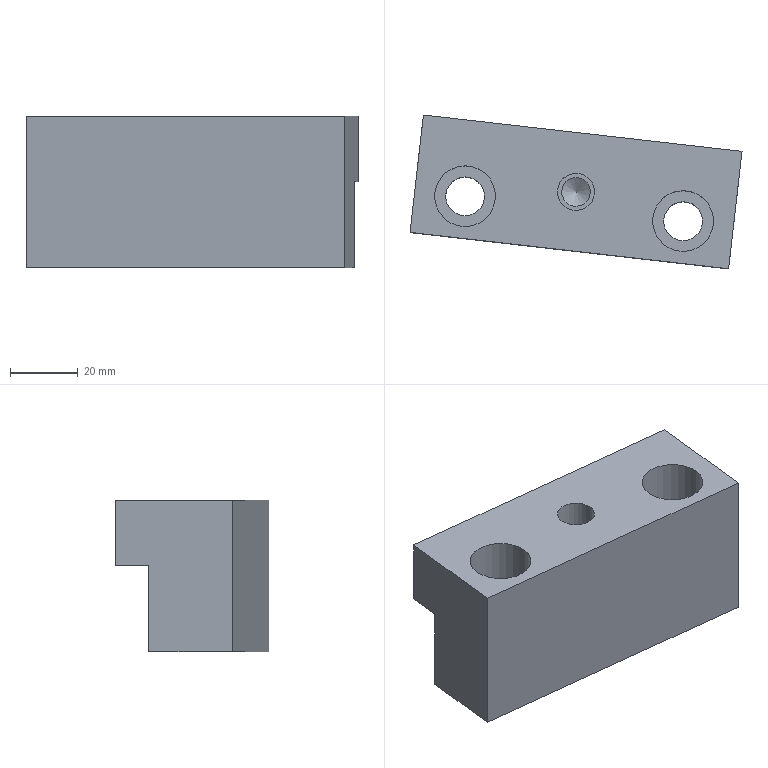Part | NX | features XQ 2 | 1 solid | 18 faces | box 98.351 x 45.529 x 45 mm | volume 108255 mm3 | plane 11 | cylinder 6 | cone 1 | commonest cylinder face diameters 11.5 x2 18 x2 8.5 x1 11 x1
STEP:
#1=CARTESIAN_POINT('',(3233.637,-396.68,-143.));
#2=VERTEX_POINT('',#1);
#3=CARTESIAN_POINT('',(3230.807,-421.519,-143.));
#4=VERTEX_POINT('',#3);
#5=CARTESIAN_POINT('',(3233.637,-396.68,-143.));
#6=DIRECTION('',(-0.1132,-0.9936,0.));
#7=VECTOR('',#6,1000.);
#8=LINE('',#5,#7);
#9=EDGE_CURVE('',#2,#4,#8,.T.);
#10=ORIENTED_EDGE('',*,*,#9,.F.);
#11=CARTESIAN_POINT('',(3328.026,-407.434,-143.));
#12=VERTEX_POINT('',#11);
#13=CARTESIAN_POINT('',(1661.613,-217.57,-143.));
#14=DIRECTION('',(-0.9936,0.1132,0.));
#15=VECTOR('',#14,1000.);
#16=LINE('',#13,#15);
#17=EDGE_CURVE('',#12,#2,#16,.T.);
#18=ORIENTED_EDGE('',*,*,#17,.F.);
#19=CARTESIAN_POINT('',(3325.196,-432.273,-143.));
#20=VERTEX_POINT('',#19);
#21=CARTESIAN_POINT('',(3342.856,-277.276,-143.));
#22=DIRECTION('',(-0.1132,-0.9936,0.));
#23=VECTOR('',#22,1000.);
#24=LINE('',#21,#23);
#25=EDGE_CURVE('',#12,#20,#24,.T.);
#26=ORIENTED_EDGE('',*,*,#25,.T.);
#27=CARTESIAN_POINT('',(1658.783,-242.409,-143.));
#28=DIRECTION('',(-0.9936,0.1132,0.));
#29=VECTOR('',#28,1000.);
#30=LINE('',#27,#29);
#31=EDGE_CURVE('',#20,#4,#30,.T.);
#32=ORIENTED_EDGE('',*,*,#31,.T.);
#33=EDGE_LOOP('',(#10,#18,#26,#32));
#34=FACE_BOUND('',#33,.T.);
#35=CARTESIAN_POINT('',(3311.708,-412.406,-143.));
#36=VERTEX_POINT('',#35);
#37=CARTESIAN_POINT('',(3311.708,-418.156,-143.));
#38=DIRECTION('',(0.,0.,-1.));
#39=DIRECTION('',(0.,1.,0.));
#40=AXIS2_PLACEMENT_3D('',#37,#38,#39);
#41=CIRCLE('',#40,5.75);
#42=EDGE_CURVE('',#36,#36,#41,.T.);
#43=ORIENTED_EDGE('',*,*,#42,.F.);
#44=EDGE_LOOP('',(#43));
#45=FACE_BOUND('',#44,.T.);
#46=CARTESIAN_POINT('',(3247.125,-405.047,-143.));
#47=VERTEX_POINT('',#46);
#48=CARTESIAN_POINT('',(3247.125,-410.797,-143.));
#49=DIRECTION('',(0.,0.,1.));
#50=DIRECTION('',(0.,1.,0.));
#51=AXIS2_PLACEMENT_3D('',#48,#49,#50);
#52=CIRCLE('',#51,5.75);
#53=EDGE_CURVE('',#47,#47,#52,.T.);
#54=ORIENTED_EDGE('',*,*,#53,.T.);
#55=EDGE_LOOP('',(#54));
#56=FACE_BOUND('',#55,.T.);
#57=CARTESIAN_POINT('',(1661.613,-217.57,-143.));
#58=DIRECTION('',(0.,0.,1.));
#59=DIRECTION('',(-0.9936,0.1132,0.));
#60=AXIS2_PLACEMENT_3D('',#57,#58,#59);
#61=PLANE('',#60);
#62=ADVANCED_FACE('',(#34,#45,#56),#61,.F.);
#63=CARTESIAN_POINT('',(3285.256,-411.071,-98.));
#64=VERTEX_POINT('',#63);
#65=CARTESIAN_POINT('',(3279.983,-409.509,-98.));
#66=DIRECTION('',(0.,0.,1.));
#67=DIRECTION('',(0.9588,-0.284,0.));
#68=AXIS2_PLACEMENT_3D('',#65,#66,#67);
#69=CIRCLE('',#68,5.5);
#70=EDGE_CURVE('',#64,#64,#69,.T.);
#71=ORIENTED_EDGE('',*,*,#70,.F.);
#72=EDGE_LOOP('',(#71));
#73=FACE_BOUND('',#72,.T.);
#74=CARTESIAN_POINT('',(3329.158,-397.498,-98.));
#75=VERTEX_POINT('',#74);
#76=CARTESIAN_POINT('',(3234.769,-386.744,-98.));
#77=VERTEX_POINT('',#76);
#78=CARTESIAN_POINT('',(3270.538,-390.819,-98.));
#79=DIRECTION('',(-0.9936,0.1132,0.));
#80=VECTOR('',#79,1000.);
#81=LINE('',#78,#80);
#82=EDGE_CURVE('',#75,#77,#81,.T.);
#83=ORIENTED_EDGE('',*,*,#82,.T.);
#84=CARTESIAN_POINT('',(3230.807,-421.519,-98.));
#85=VERTEX_POINT('',#84);
#86=CARTESIAN_POINT('',(3252.077,-234.832,-98.));
#87=DIRECTION('',(-0.1132,-0.9936,0.));
#88=VECTOR('',#87,1000.);
#89=LINE('',#86,#88);
#90=EDGE_CURVE('',#77,#85,#89,.T.);
#91=ORIENTED_EDGE('',*,*,#90,.T.);
#92=CARTESIAN_POINT('',(3325.196,-432.273,-98.));
#93=VERTEX_POINT('',#92);
#94=CARTESIAN_POINT('',(3287.44,-427.972,-98.));
#95=DIRECTION('',(-0.9936,0.1132,0.));
#96=VECTOR('',#95,1000.);
#97=LINE('',#94,#96);
#98=EDGE_CURVE('',#93,#85,#97,.T.);
#99=ORIENTED_EDGE('',*,*,#98,.F.);
#100=CARTESIAN_POINT('',(3346.466,-245.587,-98.));
#101=DIRECTION('',(-0.1132,-0.9936,0.));
#102=VECTOR('',#101,1000.);
#103=LINE('',#100,#102);
#104=EDGE_CURVE('',#75,#93,#103,.T.);
#105=ORIENTED_EDGE('',*,*,#104,.F.);
#106=EDGE_LOOP('',(#83,#91,#99,#105));
#107=FACE_BOUND('',#106,.T.);
#108=CARTESIAN_POINT('',(3311.708,-409.156,-98.));
#109=VERTEX_POINT('',#108);
#110=CARTESIAN_POINT('',(3311.708,-418.156,-98.));
#111=DIRECTION('',(0.,0.,1.));
#112=DIRECTION('',(0.,1.,0.));
#113=AXIS2_PLACEMENT_3D('',#110,#111,#112);
#114=CIRCLE('',#113,9.);
#115=EDGE_CURVE('',#109,#109,#114,.T.);
#116=ORIENTED_EDGE('',*,*,#115,.F.);
#117=EDGE_LOOP('',(#116));
#118=FACE_BOUND('',#117,.T.);
#119=CARTESIAN_POINT('',(3247.125,-401.797,-98.));
#120=VERTEX_POINT('',#119);
#121=CARTESIAN_POINT('',(3247.125,-410.797,-98.));
#122=DIRECTION('',(0.,0.,-1.));
#123=DIRECTION('',(0.,1.,0.));
#124=AXIS2_PLACEMENT_3D('',#121,#122,#123);
#125=CIRCLE('',#124,9.);
#126=EDGE_CURVE('',#120,#120,#125,.T.);
#127=ORIENTED_EDGE('',*,*,#126,.T.);
#128=EDGE_LOOP('',(#127));
#129=FACE_BOUND('',#128,.T.);
#130=CARTESIAN_POINT('',(2553.344,-155.222,-98.));
#131=DIRECTION('',(0.,0.,1.));
#132=DIRECTION('',(0.9588,-0.284,0.));
#133=AXIS2_PLACEMENT_3D('',#130,#131,#132);
#134=PLANE('',#133);
#135=ADVANCED_FACE('',(#73,#107,#118,#129),#134,.T.);
#136=CARTESIAN_POINT('',(3234.769,-386.744,-117.5));
#137=VERTEX_POINT('',#136);
#138=CARTESIAN_POINT('',(3233.637,-396.68,-117.5));
#139=VERTEX_POINT('',#138);
#140=CARTESIAN_POINT('',(3233.637,-396.68,-117.5));
#141=DIRECTION('',(-0.1132,-0.9936,0.));
#142=VECTOR('',#141,1000.);
#143=LINE('',#140,#142);
#144=EDGE_CURVE('',#137,#139,#143,.T.);
#145=ORIENTED_EDGE('',*,*,#144,.T.);
#146=CARTESIAN_POINT('',(3233.637,-396.68,-128.027));
#147=DIRECTION('',(0.,0.,1.));
#148=VECTOR('',#147,1000.);
#149=LINE('',#146,#148);
#150=EDGE_CURVE('',#2,#139,#149,.T.);
#151=ORIENTED_EDGE('',*,*,#150,.F.);
#152=ORIENTED_EDGE('',*,*,#9,.T.);
#153=CARTESIAN_POINT('',(3230.807,-421.519,-128.027));
#154=DIRECTION('',(0.,0.,1.));
#155=VECTOR('',#154,1000.);
#156=LINE('',#153,#155);
#157=EDGE_CURVE('',#4,#85,#156,.T.);
#158=ORIENTED_EDGE('',*,*,#157,.T.);
#159=ORIENTED_EDGE('',*,*,#90,.F.);
#160=CARTESIAN_POINT('',(3234.769,-386.744,-128.027));
#161=DIRECTION('',(0.,0.,1.));
#162=VECTOR('',#161,1000.);
#163=LINE('',#160,#162);
#164=EDGE_CURVE('',#137,#77,#163,.T.);
#165=ORIENTED_EDGE('',*,*,#164,.F.);
#166=EDGE_LOOP('',(#145,#151,#152,#158,#159,#165));
#167=FACE_BOUND('',#166,.T.);
#168=CARTESIAN_POINT('',(3233.637,-396.68,-128.027));
#169=DIRECTION('',(0.9936,-0.1132,0.));
#170=DIRECTION('',(0.,0.,1.));
#171=AXIS2_PLACEMENT_3D('',#168,#169,#170);
#172=PLANE('',#171);
#173=ADVANCED_FACE('',(#167),#172,.F.);
#174=CARTESIAN_POINT('',(3329.158,-397.498,-117.5));
#175=VERTEX_POINT('',#174);
#176=CARTESIAN_POINT('',(3329.158,-397.498,-118.));
#177=DIRECTION('',(0.,0.,1.));
#178=VECTOR('',#177,1000.);
#179=LINE('',#176,#178);
#180=EDGE_CURVE('',#175,#75,#179,.T.);
#181=ORIENTED_EDGE('',*,*,#180,.T.);
#182=ORIENTED_EDGE('',*,*,#104,.T.);
#183=CARTESIAN_POINT('',(3325.196,-432.273,-118.));
#184=DIRECTION('',(0.,0.,1.));
#185=VECTOR('',#184,1000.);
#186=LINE('',#183,#185);
#187=EDGE_CURVE('',#20,#93,#186,.T.);
#188=ORIENTED_EDGE('',*,*,#187,.F.);
#189=ORIENTED_EDGE('',*,*,#25,.F.);
#190=CARTESIAN_POINT('',(3328.026,-407.434,-117.5));
#191=VERTEX_POINT('',#190);
#192=CARTESIAN_POINT('',(3328.026,-407.434,-118.));
#193=DIRECTION('',(0.,0.,1.));
#194=VECTOR('',#193,1000.);
#195=LINE('',#192,#194);
#196=EDGE_CURVE('',#12,#191,#195,.T.);
#197=ORIENTED_EDGE('',*,*,#196,.T.);
#198=CARTESIAN_POINT('',(3338.113,-318.901,-117.5));
#199=DIRECTION('',(-0.1132,-0.9936,0.));
#200=VECTOR('',#199,1000.);
#201=LINE('',#198,#200);
#202=EDGE_CURVE('',#175,#191,#201,.T.);
#203=ORIENTED_EDGE('',*,*,#202,.F.);
#204=EDGE_LOOP('',(#181,#182,#188,#189,#197,#203));
#205=FACE_BOUND('',#204,.T.);
#206=CARTESIAN_POINT('',(3342.856,-277.276,-118.));
#207=DIRECTION('',(-0.9936,0.1132,0.));
#208=DIRECTION('',(-0.1132,-0.9936,0.));
#209=AXIS2_PLACEMENT_3D('',#206,#207,#208);
#210=PLANE('',#209);
#211=ADVANCED_FACE('',(#205),#210,.F.);
#212=ORIENTED_EDGE('',*,*,#187,.T.);
#213=ORIENTED_EDGE('',*,*,#98,.T.);
#214=ORIENTED_EDGE('',*,*,#157,.F.);
#215=ORIENTED_EDGE('',*,*,#31,.F.);
#216=EDGE_LOOP('',(#212,#213,#214,#215));
#217=FACE_BOUND('',#216,.T.);
#218=CARTESIAN_POINT('',(3287.44,-427.972,-88.563));
#219=DIRECTION('',(-0.1132,-0.9936,0.));
#220=DIRECTION('',(0.9936,-0.1132,0.));
#221=AXIS2_PLACEMENT_3D('',#218,#219,#220);
#222=PLANE('',#221);
#223=ADVANCED_FACE('',(#217),#222,.T.);
#224=CARTESIAN_POINT('',(2534.904,-317.069,-117.5));
#225=DIRECTION('',(-0.9936,0.1132,0.));
#226=VECTOR('',#225,1000.);
#227=LINE('',#224,#226);
#228=EDGE_CURVE('',#191,#139,#227,.T.);
#229=ORIENTED_EDGE('',*,*,#228,.F.);
#230=ORIENTED_EDGE('',*,*,#196,.F.);
#231=ORIENTED_EDGE('',*,*,#17,.T.);
#232=ORIENTED_EDGE('',*,*,#150,.T.);
#233=EDGE_LOOP('',(#229,#230,#231,#232));
#234=FACE_BOUND('',#233,.T.);
#235=CARTESIAN_POINT('',(3290.27,-403.132,-88.563));
#236=DIRECTION('',(-0.1132,-0.9936,0.));
#237=DIRECTION('',(0.9936,-0.1132,0.));
#238=AXIS2_PLACEMENT_3D('',#235,#236,#237);
#239=PLANE('',#238);
#240=ADVANCED_FACE('',(#234),#239,.F.);
#241=CARTESIAN_POINT('',(3270.538,-390.819,-117.5));
#242=DIRECTION('',(0.9936,-0.1132,0.));
#243=VECTOR('',#242,1000.);
#244=LINE('',#241,#243);
#245=EDGE_CURVE('',#137,#175,#244,.T.);
#246=ORIENTED_EDGE('',*,*,#245,.T.);
#247=ORIENTED_EDGE('',*,*,#202,.T.);
#248=ORIENTED_EDGE('',*,*,#228,.T.);
#249=ORIENTED_EDGE('',*,*,#144,.F.);
#250=EDGE_LOOP('',(#246,#247,#248,#249));
#251=FACE_BOUND('',#250,.T.);
#252=CARTESIAN_POINT('',(2544.991,-228.537,-117.5));
#253=DIRECTION('',(0.,0.,1.));
#254=DIRECTION('',(0.9981,0.06105,0.));
#255=AXIS2_PLACEMENT_3D('',#252,#253,#254);
#256=PLANE('',#255);
#257=ADVANCED_FACE('',(#251),#256,.F.);
#258=ORIENTED_EDGE('',*,*,#164,.T.);
#259=ORIENTED_EDGE('',*,*,#82,.F.);
#260=ORIENTED_EDGE('',*,*,#180,.F.);
#261=ORIENTED_EDGE('',*,*,#245,.F.);
#262=EDGE_LOOP('',(#258,#259,#260,#261));
#263=FACE_BOUND('',#262,.T.);
#264=CARTESIAN_POINT('',(3270.538,-390.819,-81.063));
#265=DIRECTION('',(-0.1132,-0.9936,0.));
#266=DIRECTION('',(0.9936,-0.1132,0.));
#267=AXIS2_PLACEMENT_3D('',#264,#265,#266);
#268=PLANE('',#267);
#269=ADVANCED_FACE('',(#263),#268,.F.);
#270=CARTESIAN_POINT('',(3311.708,-423.906,-118.));
#271=VERTEX_POINT('',#270);
#272=CARTESIAN_POINT('',(3311.708,-418.156,-118.));
#273=DIRECTION('',(0.,0.,1.));
#274=DIRECTION('',(0.,-1.,0.));
#275=AXIS2_PLACEMENT_3D('',#272,#273,#274);
#276=CIRCLE('',#275,5.75);
#277=EDGE_CURVE('',#271,#271,#276,.T.);
#278=ORIENTED_EDGE('',*,*,#277,.T.);
#279=EDGE_LOOP('',(#278));
#280=FACE_BOUND('',#279,.T.);
#281=ORIENTED_EDGE('',*,*,#42,.T.);
#282=EDGE_LOOP('',(#281));
#283=FACE_BOUND('',#282,.T.);
#284=CARTESIAN_POINT('',(3311.708,-418.156,-103.));
#285=DIRECTION('',(0.,0.,-1.));
#286=DIRECTION('',(-0.9981,-0.06105,0.));
#287=AXIS2_PLACEMENT_3D('',#284,#285,#286);
#288=CYLINDRICAL_SURFACE('',#287,5.75);
#289=ADVANCED_FACE('',(#280,#283),#288,.F.);
#290=ORIENTED_EDGE('',*,*,#277,.F.);
#291=EDGE_LOOP('',(#290));
#292=FACE_BOUND('',#291,.T.);
#293=CARTESIAN_POINT('',(3311.708,-427.156,-118.));
#294=VERTEX_POINT('',#293);
#295=CARTESIAN_POINT('',(3311.708,-418.156,-118.));
#296=DIRECTION('',(0.,0.,1.));
#297=DIRECTION('',(0.,-1.,0.));
#298=AXIS2_PLACEMENT_3D('',#295,#296,#297);
#299=CIRCLE('',#298,9.);
#300=EDGE_CURVE('',#294,#294,#299,.T.);
#301=ORIENTED_EDGE('',*,*,#300,.T.);
#302=EDGE_LOOP('',(#301));
#303=FACE_BOUND('',#302,.T.);
#304=CARTESIAN_POINT('',(3311.708,-418.156,-118.));
#305=DIRECTION('',(0.,0.,-1.));
#306=DIRECTION('',(0.9981,0.06105,0.));
#307=AXIS2_PLACEMENT_3D('',#304,#305,#306);
#308=PLANE('',#307);
#309=ADVANCED_FACE('',(#292,#303),#308,.F.);
#310=ORIENTED_EDGE('',*,*,#300,.F.);
#311=EDGE_LOOP('',(#310));
#312=FACE_BOUND('',#311,.T.);
#313=ORIENTED_EDGE('',*,*,#115,.T.);
#314=EDGE_LOOP('',(#313));
#315=FACE_BOUND('',#314,.T.);
#316=CARTESIAN_POINT('',(3311.708,-418.156,-103.));
#317=DIRECTION('',(0.,0.,-1.));
#318=DIRECTION('',(-0.9981,-0.06105,0.));
#319=AXIS2_PLACEMENT_3D('',#316,#317,#318);
#320=CYLINDRICAL_SURFACE('',#319,9.);
#321=ADVANCED_FACE('',(#312,#315),#320,.F.);
#322=CARTESIAN_POINT('',(3247.125,-416.547,-118.));
#323=VERTEX_POINT('',#322);
#324=CARTESIAN_POINT('',(3247.125,-410.797,-118.));
#325=DIRECTION('',(0.,0.,-1.));
#326=DIRECTION('',(0.,-1.,0.));
#327=AXIS2_PLACEMENT_3D('',#324,#325,#326);
#328=CIRCLE('',#327,5.75);
#329=EDGE_CURVE('',#323,#323,#328,.T.);
#330=ORIENTED_EDGE('',*,*,#329,.F.);
#331=EDGE_LOOP('',(#330));
#332=FACE_BOUND('',#331,.T.);
#333=ORIENTED_EDGE('',*,*,#53,.F.);
#334=EDGE_LOOP('',(#333));
#335=FACE_BOUND('',#334,.T.);
#336=CARTESIAN_POINT('',(3247.125,-410.797,-103.));
#337=DIRECTION('',(0.,0.,-1.));
#338=DIRECTION('',(0.9588,-0.284,0.));
#339=AXIS2_PLACEMENT_3D('',#336,#337,#338);
#340=CYLINDRICAL_SURFACE('',#339,5.75);
#341=ADVANCED_FACE('',(#332,#335),#340,.F.);
#342=ORIENTED_EDGE('',*,*,#329,.T.);
#343=EDGE_LOOP('',(#342));
#344=FACE_BOUND('',#343,.T.);
#345=CARTESIAN_POINT('',(3247.125,-419.797,-118.));
#346=VERTEX_POINT('',#345);
#347=CARTESIAN_POINT('',(3247.125,-410.797,-118.));
#348=DIRECTION('',(0.,0.,-1.));
#349=DIRECTION('',(0.,-1.,0.));
#350=AXIS2_PLACEMENT_3D('',#347,#348,#349);
#351=CIRCLE('',#350,9.);
#352=EDGE_CURVE('',#346,#346,#351,.T.);
#353=ORIENTED_EDGE('',*,*,#352,.F.);
#354=EDGE_LOOP('',(#353));
#355=FACE_BOUND('',#354,.T.);
#356=CARTESIAN_POINT('',(3247.125,-410.797,-118.));
#357=DIRECTION('',(0.,0.,-1.));
#358=DIRECTION('',(-0.9588,0.284,0.));
#359=AXIS2_PLACEMENT_3D('',#356,#357,#358);
#360=PLANE('',#359);
#361=ADVANCED_FACE('',(#344,#355),#360,.F.);
#362=ORIENTED_EDGE('',*,*,#352,.T.);
#363=EDGE_LOOP('',(#362));
#364=FACE_BOUND('',#363,.T.);
#365=ORIENTED_EDGE('',*,*,#126,.F.);
#366=EDGE_LOOP('',(#365));
#367=FACE_BOUND('',#366,.T.);
#368=CARTESIAN_POINT('',(3247.125,-410.797,-103.));
#369=DIRECTION('',(0.,0.,-1.));
#370=DIRECTION('',(0.9588,-0.284,0.));
#371=AXIS2_PLACEMENT_3D('',#368,#369,#370);
#372=CYLINDRICAL_SURFACE('',#371,9.);
#373=ADVANCED_FACE('',(#364,#367),#372,.F.);
#374=CARTESIAN_POINT('',(3274.709,-407.947,-106.));
#375=VERTEX_POINT('',#374);
#376=CARTESIAN_POINT('',(3279.983,-409.509,-106.));
#377=DIRECTION('',(0.,0.,1.));
#378=DIRECTION('',(-0.9588,0.284,0.));
#379=AXIS2_PLACEMENT_3D('',#376,#377,#378);
#380=CIRCLE('',#379,5.5);
#381=EDGE_CURVE('',#375,#375,#380,.T.);
#382=ORIENTED_EDGE('',*,*,#381,.T.);
#383=EDGE_LOOP('',(#382));
#384=FACE_BOUND('',#383,.T.);
#385=CARTESIAN_POINT('',(3275.908,-408.302,-106.));
#386=VERTEX_POINT('',#385);
#387=CARTESIAN_POINT('',(3279.983,-409.509,-106.));
#388=DIRECTION('',(0.,0.,1.));
#389=DIRECTION('',(-0.9588,0.284,0.));
#390=AXIS2_PLACEMENT_3D('',#387,#388,#389);
#391=CIRCLE('',#390,4.25);
#392=EDGE_CURVE('',#386,#386,#391,.T.);
#393=ORIENTED_EDGE('',*,*,#392,.F.);
#394=EDGE_LOOP('',(#393));
#395=FACE_BOUND('',#394,.T.);
#396=CARTESIAN_POINT('',(3279.983,-409.509,-106.));
#397=DIRECTION('',(0.,0.,-1.));
#398=DIRECTION('',(-0.9588,0.284,0.));
#399=AXIS2_PLACEMENT_3D('',#396,#397,#398);
#400=PLANE('',#399);
#401=ADVANCED_FACE('',(#384,#395),#400,.F.);
#402=ORIENTED_EDGE('',*,*,#70,.T.);
#403=EDGE_LOOP('',(#402));
#404=FACE_BOUND('',#403,.T.);
#405=ORIENTED_EDGE('',*,*,#381,.F.);
#406=EDGE_LOOP('',(#405));
#407=FACE_BOUND('',#406,.T.);
#408=CARTESIAN_POINT('',(3279.983,-409.509,-84.));
#409=DIRECTION('',(0.,0.,-1.));
#410=DIRECTION('',(-0.9588,0.284,0.));
#411=AXIS2_PLACEMENT_3D('',#408,#409,#410);
#412=CYLINDRICAL_SURFACE('',#411,5.5);
#413=ADVANCED_FACE('',(#404,#407),#412,.F.);
#414=CARTESIAN_POINT('',(3275.908,-408.302,-123.));
#415=VERTEX_POINT('',#414);
#416=CARTESIAN_POINT('',(3279.983,-409.509,-123.));
#417=DIRECTION('',(0.,0.,1.));
#418=DIRECTION('',(-0.9588,0.284,0.));
#419=AXIS2_PLACEMENT_3D('',#416,#417,#418);
#420=CIRCLE('',#419,4.25);
#421=EDGE_CURVE('',#415,#415,#420,.T.);
#422=ORIENTED_EDGE('',*,*,#421,.T.);
#423=EDGE_LOOP('',(#422));
#424=FACE_BOUND('',#423,.T.);
#425=CARTESIAN_POINT('',(3279.983,-409.509,-125.554));
#426=VERTEX_POINT('',#425);
#427=VERTEX_LOOP('',#426);
#428=FACE_BOUND('',#427,.T.);
#429=CARTESIAN_POINT('',(3279.983,-409.509,-123.));
#430=DIRECTION('',(0.,0.,1.));
#431=DIRECTION('',(0.9588,-0.284,0.));
#432=AXIS2_PLACEMENT_3D('',#429,#430,#431);
#433=CONICAL_SURFACE('',#432,4.25,1.03);
#434=ADVANCED_FACE('',(#424,#428),#433,.F.);
#435=ORIENTED_EDGE('',*,*,#392,.T.);
#436=EDGE_LOOP('',(#435));
#437=FACE_BOUND('',#436,.T.);
#438=ORIENTED_EDGE('',*,*,#421,.F.);
#439=EDGE_LOOP('',(#438));
#440=FACE_BOUND('',#439,.T.);
#441=CARTESIAN_POINT('',(3279.983,-409.509,-103.));
#442=DIRECTION('',(0.,0.,-1.));
#443=DIRECTION('',(-0.9588,0.284,0.));
#444=AXIS2_PLACEMENT_3D('',#441,#442,#443);
#445=CYLINDRICAL_SURFACE('',#444,4.25);
#446=ADVANCED_FACE('',(#437,#440),#445,.F.);
#447=CLOSED_SHELL('',(#62,#135,#173,#211,#223,#240,#257,#269,#289,#309,#321,#341,#361,#373,#401,#413,#434,#446));
#448=MANIFOLD_SOLID_BREP('',#447);
#449=(LENGTH_UNIT()NAMED_UNIT(*)SI_UNIT(.MILLI.,.METRE.));
#450=UNCERTAINTY_MEASURE_WITH_UNIT(LENGTH_MEASURE(0.00001),#449,'','');
#451=(NAMED_UNIT(*)PLANE_ANGLE_UNIT()SI_UNIT($,.RADIAN.));
#452=(NAMED_UNIT(*)SI_UNIT($,.STERADIAN.)SOLID_ANGLE_UNIT());
#453=(GEOMETRIC_REPRESENTATION_CONTEXT(3)GLOBAL_UNCERTAINTY_ASSIGNED_CONTEXT((#450))GLOBAL_UNIT_ASSIGNED_CONTEXT((#449,#451,#452))REPRESENTATION_CONTEXT('',''));
#454=ADVANCED_BREP_SHAPE_REPRESENTATION('',(#448),#453);